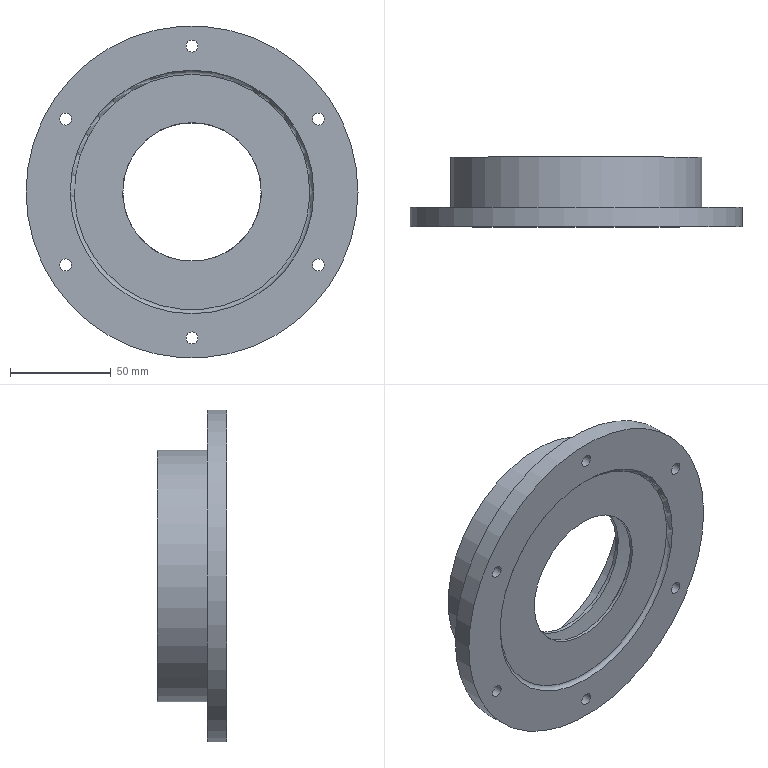Part | NX | features DATUM_CSYS 10, HOLE PACKAGE 9, SIMPLE HOLE 9, SKETCH 9, EXTRACT_DATUM_AXIS 6, EXTRACT_FACE 6, Instance Feature 5, BLEND 2, EXTRUDE 2, Pattern Feature 1, SWP104 1 | 1 solid | 21 faces | box 165 x 34.6 x 165 mm | volume 207010 mm3 | cylinder 12 | plane 5 | torus 2 | cone 2 | commonest cylinder face diameters 6 x6 69 x2 88.607 x1 116 x1 125 x1 165 x1
STEP:
#1=CARTESIAN_POINT('',(0.,-6.085,34.5));
#2=VERTEX_POINT('',#1);
#3=CARTESIAN_POINT('',(0.,-6.085,0.));
#4=DIRECTION('',(0.,1.,0.));
#5=DIRECTION('',(0.,0.,1.));
#6=AXIS2_PLACEMENT_3D('',#3,#4,#5);
#7=CIRCLE('',#6,34.5);
#8=EDGE_CURVE('',#2,#2,#7,.T.);
#9=ORIENTED_EDGE('',*,*,#8,.T.);
#10=EDGE_LOOP('',(#9));
#11=FACE_BOUND('',#10,.T.);
#12=CARTESIAN_POINT('',(0.,-7.6,34.5));
#13=VERTEX_POINT('',#12);
#14=CARTESIAN_POINT('',(0.,-7.6,0.));
#15=DIRECTION('',(0.,1.,0.));
#16=DIRECTION('',(0.,0.,1.));
#17=AXIS2_PLACEMENT_3D('',#14,#15,#16);
#18=CIRCLE('',#17,34.5);
#19=EDGE_CURVE('',#13,#13,#18,.F.);
#20=ORIENTED_EDGE('',*,*,#19,.T.);
#21=EDGE_LOOP('',(#20));
#22=FACE_BOUND('',#21,.T.);
#23=CARTESIAN_POINT('',(0.,25.,0.));
#24=DIRECTION('',(0.,-1.,0.));
#25=DIRECTION('',(0.,0.,-1.));
#26=AXIS2_PLACEMENT_3D('',#23,#24,#25);
#27=CYLINDRICAL_SURFACE('',#26,34.5);
#28=ADVANCED_FACE('',(#11,#22),#27,.F.);
#29=CARTESIAN_POINT('',(82.5,0.,0.));
#30=VERTEX_POINT('',#29);
#31=CARTESIAN_POINT('',(0.,0.,0.));
#32=DIRECTION('',(0.,-1.,0.));
#33=DIRECTION('',(1.,0.,0.));
#34=AXIS2_PLACEMENT_3D('',#31,#32,#33);
#35=CIRCLE('',#34,82.5);
#36=EDGE_CURVE('',#30,#30,#35,.T.);
#37=ORIENTED_EDGE('',*,*,#36,.T.);
#38=EDGE_LOOP('',(#37));
#39=FACE_BOUND('',#38,.T.);
#40=CARTESIAN_POINT('',(82.5,-9.6,0.));
#41=VERTEX_POINT('',#40);
#42=CARTESIAN_POINT('',(0.,-9.6,0.));
#43=DIRECTION('',(0.,-1.,0.));
#44=DIRECTION('',(1.,0.,0.));
#45=AXIS2_PLACEMENT_3D('',#42,#43,#44);
#46=CIRCLE('',#45,82.5);
#47=EDGE_CURVE('',#41,#41,#46,.T.);
#48=ORIENTED_EDGE('',*,*,#47,.F.);
#49=EDGE_LOOP('',(#48));
#50=FACE_BOUND('',#49,.T.);
#51=CARTESIAN_POINT('',(0.,0.,0.));
#52=DIRECTION('',(0.,-1.,0.));
#53=DIRECTION('',(0.,0.,-1.));
#54=AXIS2_PLACEMENT_3D('',#51,#52,#53);
#55=CYLINDRICAL_SURFACE('',#54,82.5);
#56=ADVANCED_FACE('',(#39,#50),#55,.T.);
#57=CARTESIAN_POINT('',(-62.787,0.,33.25));
#58=VERTEX_POINT('',#57);
#59=CARTESIAN_POINT('',(-62.787,0.,36.25));
#60=DIRECTION('',(0.,-1.,0.));
#61=DIRECTION('',(0.,0.,-1.));
#62=AXIS2_PLACEMENT_3D('',#59,#60,#61);
#63=CIRCLE('',#62,3.);
#64=EDGE_CURVE('',#58,#58,#63,.T.);
#65=ORIENTED_EDGE('',*,*,#64,.T.);
#66=EDGE_LOOP('',(#65));
#67=FACE_BOUND('',#66,.T.);
#68=CARTESIAN_POINT('',(-62.787,0.,-39.25));
#69=VERTEX_POINT('',#68);
#70=CARTESIAN_POINT('',(-62.787,0.,-36.25));
#71=DIRECTION('',(0.,-1.,0.));
#72=DIRECTION('',(0.,0.,-1.));
#73=AXIS2_PLACEMENT_3D('',#70,#71,#72);
#74=CIRCLE('',#73,3.);
#75=EDGE_CURVE('',#69,#69,#74,.T.);
#76=ORIENTED_EDGE('',*,*,#75,.T.);
#77=EDGE_LOOP('',(#76));
#78=FACE_BOUND('',#77,.T.);
#79=CARTESIAN_POINT('',(0.,0.,-75.5));
#80=VERTEX_POINT('',#79);
#81=CARTESIAN_POINT('',(0.,0.,-72.5));
#82=DIRECTION('',(0.,-1.,0.));
#83=DIRECTION('',(0.,0.,-1.));
#84=AXIS2_PLACEMENT_3D('',#81,#82,#83);
#85=CIRCLE('',#84,3.);
#86=EDGE_CURVE('',#80,#80,#85,.T.);
#87=ORIENTED_EDGE('',*,*,#86,.T.);
#88=EDGE_LOOP('',(#87));
#89=FACE_BOUND('',#88,.T.);
#90=CARTESIAN_POINT('',(62.787,0.,-39.25));
#91=VERTEX_POINT('',#90);
#92=CARTESIAN_POINT('',(62.787,0.,-36.25));
#93=DIRECTION('',(0.,-1.,0.));
#94=DIRECTION('',(0.,0.,-1.));
#95=AXIS2_PLACEMENT_3D('',#92,#93,#94);
#96=CIRCLE('',#95,3.);
#97=EDGE_CURVE('',#91,#91,#96,.T.);
#98=ORIENTED_EDGE('',*,*,#97,.T.);
#99=EDGE_LOOP('',(#98));
#100=FACE_BOUND('',#99,.T.);
#101=CARTESIAN_POINT('',(62.787,0.,33.25));
#102=VERTEX_POINT('',#101);
#103=CARTESIAN_POINT('',(62.787,0.,36.25));
#104=DIRECTION('',(0.,-1.,0.));
#105=DIRECTION('',(0.,0.,-1.));
#106=AXIS2_PLACEMENT_3D('',#103,#104,#105);
#107=CIRCLE('',#106,3.);
#108=EDGE_CURVE('',#102,#102,#107,.T.);
#109=ORIENTED_EDGE('',*,*,#108,.T.);
#110=EDGE_LOOP('',(#109));
#111=FACE_BOUND('',#110,.T.);
#112=CARTESIAN_POINT('',(0.,0.,69.5));
#113=VERTEX_POINT('',#112);
#114=CARTESIAN_POINT('',(0.,0.,72.5));
#115=DIRECTION('',(0.,-1.,0.));
#116=DIRECTION('',(0.,0.,-1.));
#117=AXIS2_PLACEMENT_3D('',#114,#115,#116);
#118=CIRCLE('',#117,3.);
#119=EDGE_CURVE('',#113,#113,#118,.T.);
#120=ORIENTED_EDGE('',*,*,#119,.T.);
#121=EDGE_LOOP('',(#120));
#122=FACE_BOUND('',#121,.T.);
#123=CARTESIAN_POINT('',(62.5,0.,0.));
#124=VERTEX_POINT('',#123);
#125=CARTESIAN_POINT('',(0.,0.,0.));
#126=DIRECTION('',(0.,1.,0.));
#127=DIRECTION('',(1.,0.,0.));
#128=AXIS2_PLACEMENT_3D('',#125,#126,#127);
#129=CIRCLE('',#128,62.5);
#130=EDGE_CURVE('',#124,#124,#129,.T.);
#131=ORIENTED_EDGE('',*,*,#130,.F.);
#132=EDGE_LOOP('',(#131));
#133=FACE_BOUND('',#132,.T.);
#134=ORIENTED_EDGE('',*,*,#36,.F.);
#135=EDGE_LOOP('',(#134));
#136=FACE_BOUND('',#135,.T.);
#137=CARTESIAN_POINT('',(0.,0.,0.));
#138=DIRECTION('',(0.,-1.,0.));
#139=DIRECTION('',(0.,0.,-1.));
#140=AXIS2_PLACEMENT_3D('',#137,#138,#139);
#141=PLANE('',#140);
#142=ADVANCED_FACE('',(#67,#78,#89,#100,#111,#122,#133,#136),#141,.F.);
#143=CARTESIAN_POINT('',(-62.787,-9.6,39.25));
#144=VERTEX_POINT('',#143);
#145=CARTESIAN_POINT('',(-62.787,-9.6,36.25));
#146=DIRECTION('',(0.,1.,0.));
#147=DIRECTION('',(0.,0.,1.));
#148=AXIS2_PLACEMENT_3D('',#145,#146,#147);
#149=CIRCLE('',#148,3.);
#150=EDGE_CURVE('',#144,#144,#149,.T.);
#151=ORIENTED_EDGE('',*,*,#150,.T.);
#152=EDGE_LOOP('',(#151));
#153=FACE_BOUND('',#152,.T.);
#154=CARTESIAN_POINT('',(-62.787,-9.6,-33.25));
#155=VERTEX_POINT('',#154);
#156=CARTESIAN_POINT('',(-62.787,-9.6,-36.25));
#157=DIRECTION('',(0.,1.,0.));
#158=DIRECTION('',(0.,0.,1.));
#159=AXIS2_PLACEMENT_3D('',#156,#157,#158);
#160=CIRCLE('',#159,3.);
#161=EDGE_CURVE('',#155,#155,#160,.T.);
#162=ORIENTED_EDGE('',*,*,#161,.T.);
#163=EDGE_LOOP('',(#162));
#164=FACE_BOUND('',#163,.T.);
#165=CARTESIAN_POINT('',(0.,-9.6,-69.5));
#166=VERTEX_POINT('',#165);
#167=CARTESIAN_POINT('',(0.,-9.6,-72.5));
#168=DIRECTION('',(0.,1.,0.));
#169=DIRECTION('',(0.,0.,1.));
#170=AXIS2_PLACEMENT_3D('',#167,#168,#169);
#171=CIRCLE('',#170,3.);
#172=EDGE_CURVE('',#166,#166,#171,.T.);
#173=ORIENTED_EDGE('',*,*,#172,.T.);
#174=EDGE_LOOP('',(#173));
#175=FACE_BOUND('',#174,.T.);
#176=CARTESIAN_POINT('',(62.787,-9.6,-33.25));
#177=VERTEX_POINT('',#176);
#178=CARTESIAN_POINT('',(62.787,-9.6,-36.25));
#179=DIRECTION('',(0.,1.,0.));
#180=DIRECTION('',(0.,0.,1.));
#181=AXIS2_PLACEMENT_3D('',#178,#179,#180);
#182=CIRCLE('',#181,3.);
#183=EDGE_CURVE('',#177,#177,#182,.T.);
#184=ORIENTED_EDGE('',*,*,#183,.T.);
#185=EDGE_LOOP('',(#184));
#186=FACE_BOUND('',#185,.T.);
#187=CARTESIAN_POINT('',(62.787,-9.6,39.25));
#188=VERTEX_POINT('',#187);
#189=CARTESIAN_POINT('',(62.787,-9.6,36.25));
#190=DIRECTION('',(0.,1.,0.));
#191=DIRECTION('',(0.,0.,1.));
#192=AXIS2_PLACEMENT_3D('',#189,#190,#191);
#193=CIRCLE('',#192,3.);
#194=EDGE_CURVE('',#188,#188,#193,.T.);
#195=ORIENTED_EDGE('',*,*,#194,.T.);
#196=EDGE_LOOP('',(#195));
#197=FACE_BOUND('',#196,.T.);
#198=CARTESIAN_POINT('',(0.,-9.6,75.5));
#199=VERTEX_POINT('',#198);
#200=CARTESIAN_POINT('',(0.,-9.6,72.5));
#201=DIRECTION('',(0.,1.,0.));
#202=DIRECTION('',(0.,0.,1.));
#203=AXIS2_PLACEMENT_3D('',#200,#201,#202);
#204=CIRCLE('',#203,3.);
#205=EDGE_CURVE('',#199,#199,#204,.T.);
#206=ORIENTED_EDGE('',*,*,#205,.T.);
#207=EDGE_LOOP('',(#206));
#208=FACE_BOUND('',#207,.T.);
#209=CARTESIAN_POINT('',(0.,-9.6,60.5));
#210=VERTEX_POINT('',#209);
#211=CARTESIAN_POINT('',(0.,-9.6,0.));
#212=DIRECTION('',(0.,1.,0.));
#213=DIRECTION('',(0.,0.,1.));
#214=AXIS2_PLACEMENT_3D('',#211,#212,#213);
#215=CIRCLE('',#214,60.5);
#216=EDGE_CURVE('',#210,#210,#215,.T.);
#217=ORIENTED_EDGE('',*,*,#216,.T.);
#218=EDGE_LOOP('',(#217));
#219=FACE_BOUND('',#218,.T.);
#220=ORIENTED_EDGE('',*,*,#47,.T.);
#221=EDGE_LOOP('',(#220));
#222=FACE_BOUND('',#221,.T.);
#223=CARTESIAN_POINT('',(0.,-9.6,0.));
#224=DIRECTION('',(0.,-1.,0.));
#225=DIRECTION('',(0.,0.,-1.));
#226=AXIS2_PLACEMENT_3D('',#223,#224,#225);
#227=PLANE('',#226);
#228=ADVANCED_FACE('',(#153,#164,#175,#186,#197,#208,#219,#222),#227,.T.);
#229=ORIENTED_EDGE('',*,*,#130,.T.);
#230=EDGE_LOOP('',(#229));
#231=FACE_BOUND('',#230,.T.);
#232=CARTESIAN_POINT('',(62.5,25.,0.));
#233=VERTEX_POINT('',#232);
#234=CARTESIAN_POINT('',(0.,25.,0.));
#235=DIRECTION('',(0.,1.,0.));
#236=DIRECTION('',(1.,0.,0.));
#237=AXIS2_PLACEMENT_3D('',#234,#235,#236);
#238=CIRCLE('',#237,62.5);
#239=EDGE_CURVE('',#233,#233,#238,.T.);
#240=ORIENTED_EDGE('',*,*,#239,.F.);
#241=EDGE_LOOP('',(#240));
#242=FACE_BOUND('',#241,.T.);
#243=CARTESIAN_POINT('',(0.,0.,0.));
#244=DIRECTION('',(0.,1.,0.));
#245=DIRECTION('',(0.,0.,1.));
#246=AXIS2_PLACEMENT_3D('',#243,#244,#245);
#247=CYLINDRICAL_SURFACE('',#246,62.5);
#248=ADVANCED_FACE('',(#231,#242),#247,.T.);
#249=CARTESIAN_POINT('',(0.,25.,-58.));
#250=VERTEX_POINT('',#249);
#251=CARTESIAN_POINT('',(0.,25.,0.));
#252=DIRECTION('',(0.,-1.,0.));
#253=DIRECTION('',(0.,0.,-1.));
#254=AXIS2_PLACEMENT_3D('',#251,#252,#253);
#255=CIRCLE('',#254,58.);
#256=EDGE_CURVE('',#250,#250,#255,.T.);
#257=ORIENTED_EDGE('',*,*,#256,.T.);
#258=EDGE_LOOP('',(#257));
#259=FACE_BOUND('',#258,.T.);
#260=ORIENTED_EDGE('',*,*,#239,.T.);
#261=EDGE_LOOP('',(#260));
#262=FACE_BOUND('',#261,.T.);
#263=CARTESIAN_POINT('',(0.,25.,0.));
#264=DIRECTION('',(0.,1.,0.));
#265=DIRECTION('',(0.,0.,1.));
#266=AXIS2_PLACEMENT_3D('',#263,#264,#265);
#267=PLANE('',#266);
#268=ADVANCED_FACE('',(#259,#262),#267,.T.);
#269=CARTESIAN_POINT('',(0.,4.,-53.));
#270=VERTEX_POINT('',#269);
#271=CARTESIAN_POINT('',(0.,4.,0.));
#272=DIRECTION('',(0.,-1.,0.));
#273=DIRECTION('',(0.,0.,-1.));
#274=AXIS2_PLACEMENT_3D('',#271,#272,#273);
#275=CIRCLE('',#274,53.);
#276=EDGE_CURVE('',#270,#270,#275,.F.);
#277=ORIENTED_EDGE('',*,*,#276,.T.);
#278=EDGE_LOOP('',(#277));
#279=FACE_BOUND('',#278,.T.);
#280=CARTESIAN_POINT('',(0.,4.,-34.5));
#281=VERTEX_POINT('',#280);
#282=CARTESIAN_POINT('',(0.,4.,0.));
#283=DIRECTION('',(0.,-1.,0.));
#284=DIRECTION('',(0.,0.,-1.));
#285=AXIS2_PLACEMENT_3D('',#282,#283,#284);
#286=CIRCLE('',#285,34.5);
#287=EDGE_CURVE('',#281,#281,#286,.T.);
#288=ORIENTED_EDGE('',*,*,#287,.T.);
#289=EDGE_LOOP('',(#288));
#290=FACE_BOUND('',#289,.T.);
#291=CARTESIAN_POINT('',(0.,4.,0.));
#292=DIRECTION('',(0.,-1.,0.));
#293=DIRECTION('',(0.,0.,-1.));
#294=AXIS2_PLACEMENT_3D('',#291,#292,#293);
#295=PLANE('',#294);
#296=ADVANCED_FACE('',(#279,#290),#295,.F.);
#297=CARTESIAN_POINT('',(0.,9.,-58.));
#298=VERTEX_POINT('',#297);
#299=CARTESIAN_POINT('',(0.,9.,0.));
#300=DIRECTION('',(0.,-1.,0.));
#301=DIRECTION('',(0.,0.,-1.));
#302=AXIS2_PLACEMENT_3D('',#299,#300,#301);
#303=CIRCLE('',#302,58.);
#304=EDGE_CURVE('',#298,#298,#303,.T.);
#305=ORIENTED_EDGE('',*,*,#304,.T.);
#306=EDGE_LOOP('',(#305));
#307=FACE_BOUND('',#306,.T.);
#308=ORIENTED_EDGE('',*,*,#256,.F.);
#309=EDGE_LOOP('',(#308));
#310=FACE_BOUND('',#309,.T.);
#311=CARTESIAN_POINT('',(0.,25.,0.));
#312=DIRECTION('',(0.,-1.,0.));
#313=DIRECTION('',(0.,0.,-1.));
#314=AXIS2_PLACEMENT_3D('',#311,#312,#313);
#315=CYLINDRICAL_SURFACE('',#314,58.);
#316=ADVANCED_FACE('',(#307,#310),#315,.F.);
#317=CARTESIAN_POINT('',(0.,2.322,-34.5));
#318=VERTEX_POINT('',#317);
#319=CARTESIAN_POINT('',(0.,2.322,0.));
#320=DIRECTION('',(0.,-1.,0.));
#321=DIRECTION('',(0.,0.,-1.));
#322=AXIS2_PLACEMENT_3D('',#319,#320,#321);
#323=CIRCLE('',#322,34.5);
#324=EDGE_CURVE('',#318,#318,#323,.T.);
#325=ORIENTED_EDGE('',*,*,#324,.T.);
#326=EDGE_LOOP('',(#325));
#327=FACE_BOUND('',#326,.T.);
#328=ORIENTED_EDGE('',*,*,#287,.F.);
#329=EDGE_LOOP('',(#328));
#330=FACE_BOUND('',#329,.T.);
#331=CARTESIAN_POINT('',(0.,25.,0.));
#332=DIRECTION('',(0.,-1.,0.));
#333=DIRECTION('',(0.,0.,-1.));
#334=AXIS2_PLACEMENT_3D('',#331,#332,#333);
#335=CYLINDRICAL_SURFACE('',#334,34.5);
#336=ADVANCED_FACE('',(#327,#330),#335,.F.);
#337=CARTESIAN_POINT('',(0.,-7.6,58.5));
#338=VERTEX_POINT('',#337);
#339=CARTESIAN_POINT('',(0.,-7.6,0.));
#340=DIRECTION('',(0.,1.,0.));
#341=DIRECTION('',(0.,0.,1.));
#342=AXIS2_PLACEMENT_3D('',#339,#340,#341);
#343=CIRCLE('',#342,58.5);
#344=EDGE_CURVE('',#338,#338,#343,.F.);
#345=ORIENTED_EDGE('',*,*,#344,.T.);
#346=EDGE_LOOP('',(#345));
#347=FACE_BOUND('',#346,.T.);
#348=ORIENTED_EDGE('',*,*,#19,.F.);
#349=EDGE_LOOP('',(#348));
#350=FACE_BOUND('',#349,.T.);
#351=CARTESIAN_POINT('',(0.,-7.6,0.));
#352=DIRECTION('',(0.,1.,0.));
#353=DIRECTION('',(0.,0.,1.));
#354=AXIS2_PLACEMENT_3D('',#351,#352,#353);
#355=PLANE('',#354);
#356=ADVANCED_FACE('',(#347,#350),#355,.F.);
#357=ORIENTED_EDGE('',*,*,#216,.F.);
#358=EDGE_LOOP('',(#357));
#359=FACE_BOUND('',#358,.T.);
#360=ORIENTED_EDGE('',*,*,#344,.F.);
#361=EDGE_LOOP('',(#360));
#362=FACE_BOUND('',#361,.T.);
#363=CARTESIAN_POINT('',(0.,-9.6,0.));
#364=DIRECTION('',(0.,1.,0.));
#365=DIRECTION('',(0.,0.,1.));
#366=AXIS2_PLACEMENT_3D('',#363,#364,#365);
#367=TOROIDAL_SURFACE('',#366,58.5,2.);
#368=ADVANCED_FACE('',(#359,#362),#367,.F.);
#369=CARTESIAN_POINT('',(0.,-4.882,-44.303));
#370=VERTEX_POINT('',#369);
#371=CARTESIAN_POINT('',(0.,-4.882,0.));
#372=DIRECTION('',(0.,-1.,0.));
#373=DIRECTION('',(0.,0.,-1.));
#374=AXIS2_PLACEMENT_3D('',#371,#372,#373);
#375=CIRCLE('',#374,44.303);
#376=EDGE_CURVE('',#370,#370,#375,.F.);
#377=ORIENTED_EDGE('',*,*,#376,.T.);
#378=EDGE_LOOP('',(#377));
#379=FACE_BOUND('',#378,.T.);
#380=ORIENTED_EDGE('',*,*,#8,.F.);
#381=EDGE_LOOP('',(#380));
#382=FACE_BOUND('',#381,.T.);
#383=CARTESIAN_POINT('',(0.,-7.252,0.));
#384=DIRECTION('',(0.,1.,0.));
#385=DIRECTION('',(0.,0.,1.));
#386=AXIS2_PLACEMENT_3D('',#383,#384,#385);
#387=CONICAL_SURFACE('',#386,25.,1.449);
#388=ADVANCED_FACE('',(#379,#382),#387,.F.);
#389=CARTESIAN_POINT('',(0.,1.118,-44.303));
#390=VERTEX_POINT('',#389);
#391=CARTESIAN_POINT('',(0.,1.118,0.));
#392=DIRECTION('',(0.,-1.,0.));
#393=DIRECTION('',(0.,0.,-1.));
#394=AXIS2_PLACEMENT_3D('',#391,#392,#393);
#395=CIRCLE('',#394,44.303);
#396=EDGE_CURVE('',#390,#390,#395,.F.);
#397=ORIENTED_EDGE('',*,*,#396,.F.);
#398=EDGE_LOOP('',(#397));
#399=FACE_BOUND('',#398,.T.);
#400=ORIENTED_EDGE('',*,*,#324,.F.);
#401=EDGE_LOOP('',(#400));
#402=FACE_BOUND('',#401,.T.);
#403=CARTESIAN_POINT('',(0.,1.118,0.));
#404=DIRECTION('',(0.,-1.,0.));
#405=DIRECTION('',(0.,0.,-1.));
#406=AXIS2_PLACEMENT_3D('',#403,#404,#405);
#407=CONICAL_SURFACE('',#406,44.303,1.449);
#408=ADVANCED_FACE('',(#399,#402),#407,.F.);
#409=ORIENTED_EDGE('',*,*,#396,.T.);
#410=EDGE_LOOP('',(#409));
#411=FACE_BOUND('',#410,.T.);
#412=ORIENTED_EDGE('',*,*,#376,.F.);
#413=EDGE_LOOP('',(#412));
#414=FACE_BOUND('',#413,.T.);
#415=CARTESIAN_POINT('',(0.,-9.6,0.));
#416=DIRECTION('',(0.,-1.,0.));
#417=DIRECTION('',(0.,0.,-1.));
#418=AXIS2_PLACEMENT_3D('',#415,#416,#417);
#419=CYLINDRICAL_SURFACE('',#418,44.303);
#420=ADVANCED_FACE('',(#411,#414),#419,.F.);
#421=ORIENTED_EDGE('',*,*,#304,.F.);
#422=EDGE_LOOP('',(#421));
#423=FACE_BOUND('',#422,.T.);
#424=ORIENTED_EDGE('',*,*,#276,.F.);
#425=EDGE_LOOP('',(#424));
#426=FACE_BOUND('',#425,.T.);
#427=CARTESIAN_POINT('',(0.,9.,0.));
#428=DIRECTION('',(0.,-1.,0.));
#429=DIRECTION('',(0.,0.,-1.));
#430=AXIS2_PLACEMENT_3D('',#427,#428,#429);
#431=TOROIDAL_SURFACE('',#430,53.,5.);
#432=ADVANCED_FACE('',(#423,#426),#431,.F.);
#433=ORIENTED_EDGE('',*,*,#205,.F.);
#434=EDGE_LOOP('',(#433));
#435=FACE_BOUND('',#434,.T.);
#436=ORIENTED_EDGE('',*,*,#119,.F.);
#437=EDGE_LOOP('',(#436));
#438=FACE_BOUND('',#437,.T.);
#439=CARTESIAN_POINT('',(0.,-9.6,72.5));
#440=DIRECTION('',(0.,1.,0.));
#441=DIRECTION('',(0.,0.,1.));
#442=AXIS2_PLACEMENT_3D('',#439,#440,#441);
#443=CYLINDRICAL_SURFACE('',#442,3.);
#444=ADVANCED_FACE('',(#435,#438),#443,.F.);
#445=ORIENTED_EDGE('',*,*,#194,.F.);
#446=EDGE_LOOP('',(#445));
#447=FACE_BOUND('',#446,.T.);
#448=ORIENTED_EDGE('',*,*,#108,.F.);
#449=EDGE_LOOP('',(#448));
#450=FACE_BOUND('',#449,.T.);
#451=CARTESIAN_POINT('',(62.787,-9.6,36.25));
#452=DIRECTION('',(0.,1.,0.));
#453=DIRECTION('',(0.,0.,1.));
#454=AXIS2_PLACEMENT_3D('',#451,#452,#453);
#455=CYLINDRICAL_SURFACE('',#454,3.);
#456=ADVANCED_FACE('',(#447,#450),#455,.F.);
#457=ORIENTED_EDGE('',*,*,#183,.F.);
#458=EDGE_LOOP('',(#457));
#459=FACE_BOUND('',#458,.T.);
#460=ORIENTED_EDGE('',*,*,#97,.F.);
#461=EDGE_LOOP('',(#460));
#462=FACE_BOUND('',#461,.T.);
#463=CARTESIAN_POINT('',(62.787,-9.6,-36.25));
#464=DIRECTION('',(0.,1.,0.));
#465=DIRECTION('',(0.,0.,1.));
#466=AXIS2_PLACEMENT_3D('',#463,#464,#465);
#467=CYLINDRICAL_SURFACE('',#466,3.);
#468=ADVANCED_FACE('',(#459,#462),#467,.F.);
#469=ORIENTED_EDGE('',*,*,#172,.F.);
#470=EDGE_LOOP('',(#469));
#471=FACE_BOUND('',#470,.T.);
#472=ORIENTED_EDGE('',*,*,#86,.F.);
#473=EDGE_LOOP('',(#472));
#474=FACE_BOUND('',#473,.T.);
#475=CARTESIAN_POINT('',(0.,-9.6,-72.5));
#476=DIRECTION('',(0.,1.,0.));
#477=DIRECTION('',(0.,0.,1.));
#478=AXIS2_PLACEMENT_3D('',#475,#476,#477);
#479=CYLINDRICAL_SURFACE('',#478,3.);
#480=ADVANCED_FACE('',(#471,#474),#479,.F.);
#481=ORIENTED_EDGE('',*,*,#161,.F.);
#482=EDGE_LOOP('',(#481));
#483=FACE_BOUND('',#482,.T.);
#484=ORIENTED_EDGE('',*,*,#75,.F.);
#485=EDGE_LOOP('',(#484));
#486=FACE_BOUND('',#485,.T.);
#487=CARTESIAN_POINT('',(-62.787,-9.6,-36.25));
#488=DIRECTION('',(0.,1.,0.));
#489=DIRECTION('',(0.,0.,1.));
#490=AXIS2_PLACEMENT_3D('',#487,#488,#489);
#491=CYLINDRICAL_SURFACE('',#490,3.);
#492=ADVANCED_FACE('',(#483,#486),#491,.F.);
#493=ORIENTED_EDGE('',*,*,#150,.F.);
#494=EDGE_LOOP('',(#493));
#495=FACE_BOUND('',#494,.T.);
#496=ORIENTED_EDGE('',*,*,#64,.F.);
#497=EDGE_LOOP('',(#496));
#498=FACE_BOUND('',#497,.T.);
#499=CARTESIAN_POINT('',(-62.787,-9.6,36.25));
#500=DIRECTION('',(0.,1.,0.));
#501=DIRECTION('',(0.,0.,1.));
#502=AXIS2_PLACEMENT_3D('',#499,#500,#501);
#503=CYLINDRICAL_SURFACE('',#502,3.);
#504=ADVANCED_FACE('',(#495,#498),#503,.F.);
#505=CLOSED_SHELL('',(#28,#56,#142,#228,#248,#268,#296,#316,#336,#356,#368,#388,#408,#420,#432,#444,#456,#468,#480,#492,#504));
#506=MANIFOLD_SOLID_BREP('',#505);
#507=(LENGTH_UNIT()NAMED_UNIT(*)SI_UNIT(.MILLI.,.METRE.));
#508=UNCERTAINTY_MEASURE_WITH_UNIT(LENGTH_MEASURE(0.00001),#507,'','');
#509=(NAMED_UNIT(*)PLANE_ANGLE_UNIT()SI_UNIT($,.RADIAN.));
#510=(NAMED_UNIT(*)SI_UNIT($,.STERADIAN.)SOLID_ANGLE_UNIT());
#511=(GEOMETRIC_REPRESENTATION_CONTEXT(3)GLOBAL_UNCERTAINTY_ASSIGNED_CONTEXT((#508))GLOBAL_UNIT_ASSIGNED_CONTEXT((#507,#509,#510))REPRESENTATION_CONTEXT('',''));
#512=ADVANCED_BREP_SHAPE_REPRESENTATION('',(#506),#511);